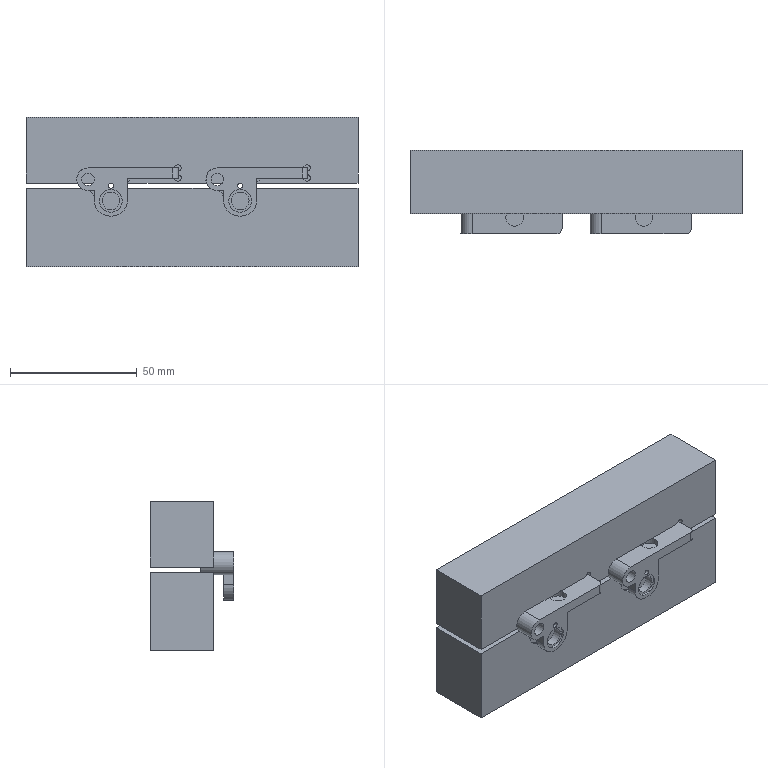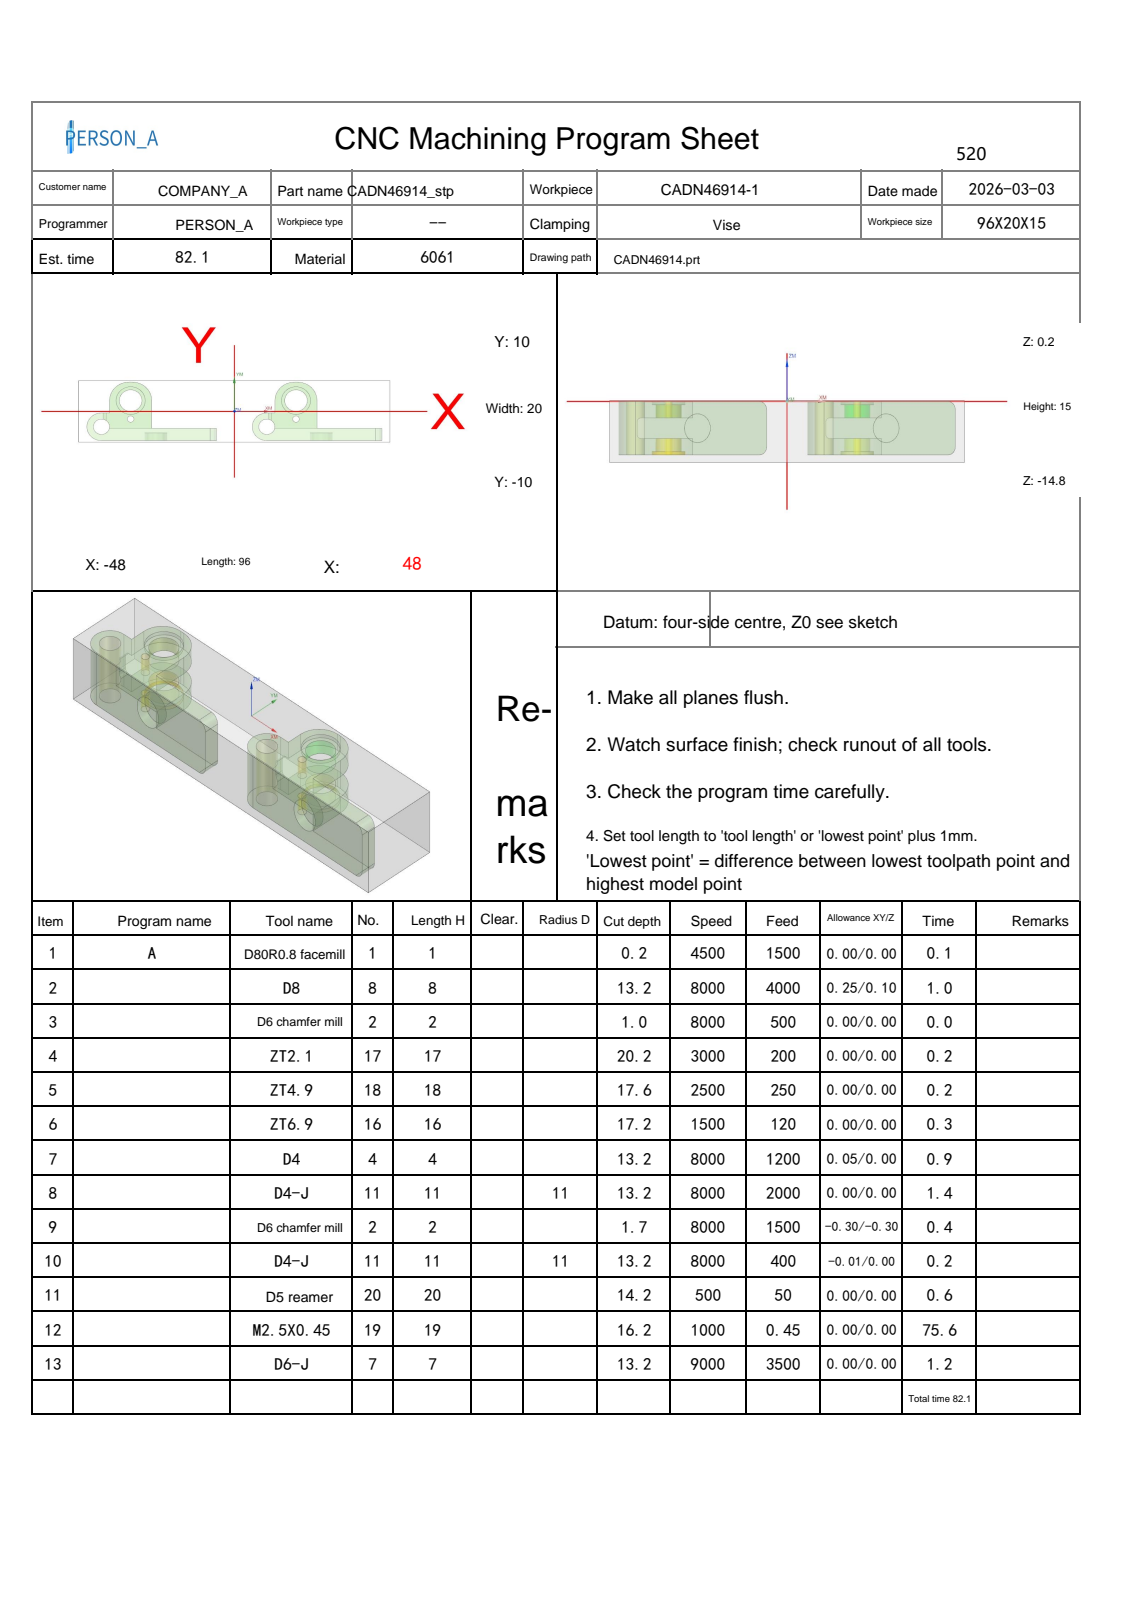NC program | NX | posted by the shop | part box 131 x 33 x 59 mm
Lines 9140 to 10309 of 12027:
N13 T07 M06
(D6-J  D=6. R=0. H=07 ce=0.01 di=0.00)
G00 G90 G54 X46.649 Y.748 M03 S7000
G43 H07 Z10.2
M08
Z.492
G01 Z-.008 F3500.
X46.545 Y-4.398
G02 X46.689 Y-5.5 I-16.56 J-2.717
G01 Y-9.5
G02 X46.536 Y-10.609 I-18.771 J2.023
G01 X46.578 Y-10.607 Z-.012
X46.729 Y-9.5
Y-5.5
G03 X46.592 Y-4.399 I-822.675 J-101.969
G01 X46.63 Y-4.4 Z-.016
G03 X46.738 Y-5.181 I4.184 J.179
G01 X46.707 Y-5.189
X46.762 Y-5.5
Y-9.5
X46.619 Y-10.601
X46.64 Y-10.6 Z-.02
X46.695 Y-10.135
X46.72 Y-10.074
X46.792 Y-9.5
Y-5.5
X46.735 Y-5.189
X46.752 Y-5.201
X46.77 Y-5.19
X46.767 Y-5.17
X46.758 Y-5.109
G02 X46.653 Y-4.4 I3.354 J.858
G01 X46.675 Z-.024
X46.674 Y-4.451
G03 X46.729 Y-4.821 I1.275 J0.0
G01 X46.715 Y-4.848
X46.75 Y-4.874
X46.802 Y-5.178
X46.764 Y-5.189
X46.819 Y-5.5
Y-9.5
G02 X46.736 Y-10.108 I-2.526 J.034
G01 X46.722 Y-10.122
X46.658 Y-10.601
X46.675 Z-.028
X46.751 Y-10.206
X46.742 Y-10.141
X46.781 Y-10.086
X46.802 Y-10.022
X46.803 Y-9.954
X46.843 Y-9.5
Y-5.5
X46.792 Y-5.189
X46.826 Y-5.177
X46.819 Y-5.167
X46.775 Y-4.873
X46.742
X46.73 Y-4.837
X46.757 Y-4.818
G02 X46.697 Y-4.449 I1.094 J.369
G01 X46.698 Y-4.4
X46.721 Z-.032
X46.719 Y-4.447
G03 X46.785 Y-4.815 I1.055 J0.0
G01 X46.754 Y-4.83
X46.761 Y-4.868
X46.795 Y-4.872
X46.839 Y-5.166
X46.849 Y-5.176
X46.82 Y-5.189
X46.866 Y-5.5
Y-9.5
G02 X46.809 Y-10.084 I-5.205 J.215
G01 X46.766 Y-10.143
X46.778 Y-10.209
X46.693 Y-10.601
X46.71 Y-10.602 Z-.036
X46.801 Y-10.211
X46.78 Y-10.188
X46.777 Y-10.157
X46.794 Y-10.13
X46.818 Y-10.117
G03 X46.888 Y-9.5 I-2.923 J.644
G01 Y-5.5
X46.849 Y-5.189
X46.858 Y-5.193
X46.865 Y-5.185
X46.861 Y-5.176
X46.815 Y-4.871
X46.783 Y-4.864
X46.777 Y-4.829
X46.805 Y-4.812
G02 X46.743 Y-4.416 I1.229 J.396
G01 Y-4.399
X46.765 Z-.038
X46.766 Z-.04
G03 X46.822 Y-4.81 I1.682 J.022
G01 X46.799 Y-4.83
X46.805 Y-4.862
X46.835 Y-4.87
G02 X46.908 Y-5.5 I-4.491 J-.843
G01 Y-9.5
G02 X46.843 Y-10.12 I-3.998 J.106
G01 X46.824 Y-10.115
X46.809 Y-10.129
X46.813 Y-10.148
X46.817 Y-10.213
X46.728 Y-10.602
X46.744 Z-.044
G03 X46.913 Y-9.785 I-8.742 J2.237
G01 X46.927 Y-9.5
Y-5.5
G03 X46.862 Y-4.936 I-2.943 J-.055
G02 X46.788 Y-4.399 I2.404 J.604
G01 X46.802 Z-.046
X46.805 Z-.048
Y-4.404
G03 X46.855 Y-4.803 I1.626 J0.0
G02 X46.946 Y-5.5 I-2.862 J-.726
G01 Y-9.5
G02 X46.761 Y-10.602 I-4.616 J.208
G01 X46.777 Z-.052
X46.895 Y-10.099
G03 X46.963 Y-9.514 I-2.488 J.584
G01 Y-5.5
G03 X46.873 Y-4.805 I-2.886 J-.021
G02 X46.82 Y-4.434 I1.262 J.371
G01 Y-4.399
X46.835 Z-.056
X46.834 Y-4.435
G03 X46.89 Y-4.803 I1.252 J0.0
G02 X46.98 Y-5.496 I-2.615 J-.693
G01 Y-5.5
Y-9.5
G02 X46.907 Y-10.159 I-3.404 J.044
G01 X46.884 Y-10.22
X46.865 Y-10.298
X46.794 Y-10.602
X46.81 Z-.06
X46.9 Y-10.222
X46.925 Y-10.145
G03 X46.996 Y-9.5 I-3.369 J.697
G01 Y-5.5
Y-5.499
G03 X46.872 Y-4.673 I-2.806 J0.0
G01 X46.85 Y-4.4
X46.865 Z-.064
X46.864 Y-4.439
G03 X46.923 Y-4.799 I1.119 J0.0
G01 X46.94 Y-4.848
G02 X47.012 Y-5.5 I-3.583 J-.726
G01 Y-9.5
G02 X46.941 Y-10.146 I-3.831 J.095
G01 X46.917 Y-10.224
X46.827 Y-10.602
X46.843 Z-.068
G03 X47.027 Y-9.5 I-4.589 J1.332
G01 Y-5.477
G03 X46.919 Y-4.724 I-2.67 J0.0
G02 X46.879 Y-4.443 I.959 J.281
G01 Y-4.4
X46.894 Z-.072
Y-4.432
G03 X46.929 Y-4.688 I.946 J0.0
G02 X47.042 Y-5.5 I-3.368 J-.881
G01 Y-9.5
G02 X46.86 Y-10.602 I-4.792 J.225
G01 X46.876 Z-.076
G03 X47.056 Y-9.5 I-4.798 J1.348
G01 Y-5.5
G03 X46.965 Y-4.765 I-4.457 J-.18
G01 X46.958 Y-4.744
G02 X46.908 Y-4.441 I.887 J.303
G01 X46.909 Y-4.4
X46.924 Z-.08
Y-4.423
G03 X46.951 Y-4.655 I.983 J0.0
G02 X47.07 Y-5.5 I-4.213 J-1.022
G01 Y-9.5
G02 X46.893 Y-10.602 I-5.338 J.293
G01 X46.909 Z-.084
G03 X47.084 Y-9.5 I-5.534 J1.439
G01 Y-5.5
G03 X46.974 Y-4.706 I-4.032 J-.151
G02 X46.939 Y-4.418 I1.159 J.289
G01 Y-4.4
X46.953 Z-.086
X46.954 Z-.088
G03 X47.006 Y-4.786 I1.493 J.003
G02 X47.097 Y-5.5 I-3.649 J-.829
G01 Y-9.5
X47.055 Y-9.957
X46.926 Y-10.602
X46.942 Y-10.601 Z-.092
X47.063 Y-9.983
G03 X47.11 Y-9.507 I-2.419 J.476
G01 Y-5.5
G03 X47.005 Y-4.745 I-3.431 J-.089
G02 X46.967 Y-4.442 I1.193 J.303
G01 X46.968 Y-4.4
X46.977 Z-.094
X46.979 Z-.096
X46.978 Y-4.444
G03 X47.017 Y-4.749 I1.188 J0.0
G02 X47.122 Y-5.5 I-3.055 J-.809
G01 Y-9.501
G02 X47.073 Y-9.999 I-2.565 J0.0
G01 X46.965 Y-10.547
X46.957 Y-10.601
X46.973 Z-.1
G02 X47.076 Y-10.038 I6.185 J-.841
G03 X47.135 Y-9.522 I-2.236 J.516
G01 Y-5.5
G03 X47.03 Y-4.753 I-2.912 J-.027
G02 X46.989 Y-4.449 I1.102 J.304
G01 X46.99 Y-4.4
X47.001 Z-.104
X46.999 Y-4.455
G03 X47.041 Y-4.754 I1.082 J0.0
G02 X47.147 Y-5.5 I-2.611 J-.749
G01 Y-9.552
G02 X47.09 Y-10.032 I-2.062 J0.0
G03 X46.985 Y-10.601 I5.359 J-1.284
G01 X46.987 Z-.106
X46.997 Z-.108
G02 X47.097 Y-10.053 I4.944 J-.626
G03 X47.158 Y-9.542 I-2.112 J.512
G01 Y-5.5
Y-5.498
G03 X47.053 Y-4.756 I-2.658 J0.0
G02 X47.01 Y-4.457 I1.027 J.299
G01 X47.012 Y-4.4
X47.023 Z-.112
X47.02 Y-4.468
G03 X47.062 Y-4.75 I.964 J0.0
G02 X47.17 Y-5.474 I-2.372 J-.724
G01 Y-5.5
Y-9.5
G02 X47.135 Y-9.957 I-4.923 J.146
G03 X47.009 Y-10.601 I4.41 J-1.201
G01 X47.021 Z-.116
G02 X47.146 Y-9.957 I4.894 J-.613
G03 X47.182 Y-9.5 I-5.306 J.652
G01 Y-5.5
G03 X47.099 Y-4.848 I-2.646 J-.007
G01 X47.097 Y-4.768
X47.057 Y-4.697
G02 X47.034 Y-4.404 I1.898 J.293
G01 Y-4.4
X47.046 Z-.121
X47.068 Y-4.696
X47.102 Y-4.776
X47.111 Y-4.848
X47.164 Y-5.135
G02 X47.194 Y-5.469 I-1.826 J-.333
G01 Y-9.51
G02 X47.13 Y-10.064 I-2.444 J0.0
G03 X47.034 Y-10.601 I5.243 J-1.219
G01 X47.047 Z-.125
G02 X47.144 Y-10.056 I5.891 J-.768
G03 X47.206 Y-9.503 I-2.442 J.553
G01 Y-5.5
Y-5.476
G03 X47.185 Y-5.189 I-1.947 J0.0
G01 X47.124 Y-4.848
X47.114 Y-4.774
X47.079 Y-4.695
X47.058 Y-4.4
X47.07 Z-.129
X47.09 Y-4.694
X47.127 Y-4.773
X47.137 Y-4.848
X47.196 Y-5.189
G02 X47.218 Y-5.475 I-1.87 J-.286
G01 Y-5.5
Y-9.505
G02 X47.158 Y-10.043 I-2.469 J0.0
G03 X47.06 Y-10.601 I6.131 J-1.369
G01 X47.071 Z-.132
X47.073 Z-.134
G02 X47.173 Y-10.029 I7.441 J-1.009
G03 X47.229 Y-9.504 I-2.438 J.525
G01 Y-5.5
Y-5.479
G03 X47.207 Y-5.189 I-1.927 J0.0
G01 X47.15 Y-4.848
X47.139 Y-4.772
X47.102 Y-4.692
X47.082 Y-4.4
X47.095 Z-.138
X47.113 Y-4.691
X47.143 Y-4.732
X47.148 Y-4.783
G02 X47.241 Y-5.5 I-3.31 J-.792
G01 Y-9.505
G02 X47.188 Y-10.015 I-2.493 J0.0
G03 X47.086 Y-10.601 I8.476 J-1.771
G01 X47.099 Z-.143
X47.143 Y-10.298
X47.171 Y-10.173
G03 X47.252 Y-9.5 I-3.724 J.788
G01 Y-5.5
G03 X47.163 Y-4.79 I-3.575 J-.086
G01 X47.157 Y-4.735
X47.124 Y-4.69
X47.107 Y-4.4
X47.119 Z-.147
X47.136 Y-4.689
X47.178 Y-4.763
X47.189 Y-4.848
G02 X47.263 Y-5.5 I-3.658 J-.745
G01 Y-9.503
G02 X47.165 Y-10.254 I-2.937 J0.0
G01 X47.154 Y-10.298
X47.112 Y-10.601
X47.126 Z-.152
X47.165 Y-10.298
X47.183 Y-10.237
G03 X47.275 Y-9.5 I-3.818 J.848
G01 Y-5.5
G03 X47.203 Y-4.848 I-3.879 J-.096
G01 X47.18 Y-4.767
X47.148 Y-4.687
G02 X47.132 Y-4.4 I3.666 J.345
G01 X47.146 Z-.157
X47.154 Y-4.638
X47.175 Y-4.712
G02 X47.287 Y-5.496 I-2.696 J-.785
G01 Y-9.5
G02 X47.195 Y-10.238 I-3.778 J.094
G01 X47.176 Y-10.298
X47.141 Y-10.6
X47.156 Z-.162
X47.188 Y-10.298
X47.208 Y-10.239
G03 X47.299 Y-9.5 I-3.54 J.813
G01 Y-5.451
G03 X47.202 Y-4.765 I-2.483 J0.0
G02 X47.158 Y-4.476 I.907 J.289
G01 X47.161 Y-4.4
X47.175 Z-.168
X47.188 Y-4.683
G02 X47.312 Y-5.475 I-2.476 J-.792
G01 X47.311 Y-5.5
Y-9.5
G02 X47.221 Y-10.24 I-3.466 J.05
G01 X47.2 Y-10.298
X47.172 Y-10.6
X47.188 Z-.173
X47.213 Y-10.298
G03 X47.324 Y-9.5 I-2.862 J.804
G01 Y-5.5
Y-5.477
G03 X47.202 Y-4.681 I-2.654 J0.0
G01 X47.19 Y-4.4
X47.205 Z-.179
X47.216 Y-4.68
G02 X47.336 Y-5.496 I-2.713 J-.816
G01 Y-5.5
Y-9.5
Y-9.508
G02 X47.226 Y-10.298 I-2.876 J0.0
G01 X47.204 Y-10.6
X47.22 Z-.184
X47.239 Y-10.298
G03 X47.349 Y-9.5 I-2.994 J.819
G01 Y-5.5
G03 X47.25 Y-4.739 I-3.274 J-.037
G02 X47.218 Y-4.479 I1.037 J.26
G01 X47.221 Y-4.4
X47.237 Z-.19
X47.235 Y-4.472
G03 X47.275 Y-4.802 I1.366 J0.0
G02 X47.361 Y-5.5 I-2.812 J-.7
G01 Y-9.5
G02 X47.269 Y-10.234 I-3.542 J.069
G03 X47.235 Y-10.533 I1.284 J-.299
G01 X47.237 Y-10.6
X47.254 Z-.196
X47.25 Y-10.511
G02 X47.28 Y-10.247 I1.194 J0.0
G03 X47.373 Y-9.5 I-3.736 J.846
G01 Y-5.5
G03 X47.284 Y-4.773 I-3.481 J-.058
G02 X47.25 Y-4.478 I1.279 J.296
G01 X47.253 Y-4.4
X47.269 Z-.202
X47.267 Y-4.478
G03 X47.302 Y-4.81 I1.582 J0.0
G02 X47.385 Y-5.5 I-3.736 J-.801
G01 Y-9.5
G02 X47.287 Y-10.276 I-4.279 J.147
G03 X47.264 Y-10.487 I.961 J-.212
G01 X47.271 Y-10.6
X47.288 Z-.208
X47.292 Y-10.298
G03 X47.398 Y-9.5 I-3.987 J.932
G01 Y-5.5
G03 X47.316 Y-4.813 I-4.303 J-.165
G02 X47.283 Y-4.487 I1.612 J.326
G01 X47.285 Y-4.4
X47.301 Z-.211
X47.306 Z-.214
X47.305 Y-4.464
G03 X47.354 Y-4.943 I2.393 J0.0
G01 X47.41 Y-5.5
Y-9.5
G02 X47.325 Y-10.2 I-4.378 J.175
G03 X47.295 Y-10.449 I1.025 J-.249
G01 X47.306 Y-10.6
X47.318 Z-.22
X47.307 Y-10.45
G02 X47.336 Y-10.201 I1.076 J0.0
G03 X47.422 Y-9.5 I-4.237 J.876
G01 Y-5.5
X47.375 Y-5.027
X47.365 Y-4.942
G02 X47.315 Y-4.421 I2.673 J.521
G01 Y-4.4
X47.324 Z-.223
X47.327 Z-.227
Y-4.428
G03 X47.377 Y-4.941 I2.639 J0.0
G01 X47.386 Y-5.026
X47.435 Y-5.5
Y-9.5
G02 X47.348 Y-10.202 I-4.222 J.167
G03 X47.319 Y-10.45 I1.07 J-.247
G01 X47.33 Y-10.6
X47.342 Z-.233
X47.332 Y-10.45
G02 X47.359 Y-10.203 I1.123 J0.0
G03 X47.447 Y-9.5 I-4.003 J.857
G01 Y-5.5
X47.397 Y-5.025
X47.389 Y-4.941
G02 X47.339 Y-4.435 I2.507 J.506
G01 Y-4.4
X47.348 Z-.236
X47.351 Z-.24
G03 X47.43 Y-5.189 I7.637 J.36
G01 X47.459 Y-5.5
Y-9.5
G02 X47.371 Y-10.204 I-3.936 J.137
G03 X47.344 Y-10.45 I1.123 J-.246
G01 X47.354 Y-10.6
X47.366 Z-.246
X47.357 Y-10.45
G02 X47.383 Y-10.205 I1.179 J0.0
G03 X47.471 Y-9.5 I-3.696 J.824
G01 Y-5.5
X47.442 Y-5.189
G02 X47.364 Y-4.4 I7.656 J1.157
G01 X47.373 Z-.25
X47.376 Z-.253
G03 X47.454 Y-5.189 I7.872 J.379
G01 X47.483 Y-5.5
Y-9.5
G02 X47.394 Y-10.206 I-3.788 J.119
G03 X47.37 Y-10.45 I1.186 J-.244
G01 X47.379 Y-10.6
X47.392 Z-.26
X47.382 Y-10.449
G02 X47.428 Y-10.118 I1.212 J0.0
X47.482 Y-9.778 I2.42 J-.208
G01 X47.496 Y-9.5
Y-5.5
X47.467 Y-5.189
G02 X47.389 Y-4.4 I7.949 J1.181
G01 X47.398 Z-.263
X47.402 Z-.267
G03 X47.508 Y-5.5 I22.285 J1.585
G01 Y-9.5
G02 X47.419 Y-10.208 I-3.811 J.119
G03 X47.396 Y-10.45 I1.263 J-.242
G01 X47.405 Y-10.6
X47.418 Z-.274
X47.409 Y-10.45
G02 X47.431 Y-10.209 I1.33 J0.0
G03 X47.52 Y-9.5 I-3.868 J.843
G01 Y-5.5
X47.493 Y-5.189
G02 X47.415 Y-4.4 I8.233 J1.205
G01 X47.425 Z-.277
X47.428 Z-.281
G03 X47.506 Y-5.189 I8.509 J.433
G01 X47.532 Y-5.5
Y-9.5
G02 X47.444 Y-10.21 I-4.097 J.147
G03 X47.423 Y-10.45 I1.358 J-.24
G01 X47.431 Y-10.6
X47.444 Z-.288
X47.437 Y-10.45
G02 X47.457 Y-10.211 I1.434 J0.0
G03 X47.544 Y-9.5 I-4.186 J.874
G01 Y-5.5
G03 X47.508 Y-5.118 I-3.844 J-.162
G02 X47.442 Y-4.4 I7.221 J1.032
G01 X47.451 Z-.291
X47.455 Z-.295
X47.483 Y-4.848
G02 X47.555 Y-5.5 I-5.164 J-.9
G01 Y-9.5
G02 X47.475 Y-10.182 I-4.26 J.155
G03 X47.449 Y-10.447 I1.327 J-.266
G01 X47.458 Y-10.6
X47.471 Z-.302
X47.464 Y-10.45
G02 X47.498 Y-10.124 I1.549 J0.0
G03 X47.567 Y-9.5 I-4.31 J.788
G01 Y-5.5
G03 X47.494 Y-4.848 I-4.534 J-.176
G01 X47.468 Y-4.4
X47.478 Z-.306
X47.481 Z-.309
X47.505 Y-4.848
G02 X47.578 Y-5.5 I-3.894 J-.768
G01 Y-9.5
G02 X47.509 Y-10.124 I-4.041 J.132
G03 X47.477 Y-10.452 I1.645 J-.328
G01 X47.483 Y-10.6
X47.491 Z-.313
X47.495 Z-.316
X47.489 Y-10.459
G02 X47.519 Y-10.141 I1.707 J0.0
G03 X47.589 Y-9.5 I-4.09 J.774
G01 Y-5.5
G03 X47.516 Y-4.848 I-3.503 J-.067
G01 X47.493 Y-4.4
X47.504 Z-.32
X47.505 Z-.323
X47.526 Y-4.848
G02 X47.6 Y-5.5 I-3.043 J-.676
G01 Y-9.5
G02 X47.529 Y-10.16 I-4.302 J.133
G03 X47.501 Y-10.462 I1.611 J-.302
G01 X47.506 Y-10.6
X47.518 Z-.327
Z-.331
X47.514 Y-10.465
G02 X47.541 Y-10.127 I2.111 J0.0
G01 X47.562 Y-10.042
X47.576 Y-9.957
X47.612 Y-9.5
Y-5.5
G03 X47.537 Y-4.848 I-2.966 J-.008
G01 X47.518 Y-4.4
X47.532 Z-.335
X47.531 Z-.339
X47.549 Y-4.848
G02 X47.623 Y-5.5 I-2.832 J-.652
G01 Y-9.5
X47.588 Y-9.957
X47.574 Y-10.043
X47.553 Y-10.128
G03 X47.529 Y-10.495 I2.818 J-.367
G01 X47.531 Y-10.6
X47.547 Z-.343
X47.544 Z-.347
X47.541 Y-10.488
G02 X47.585 Y-10.044 I2.294 J0.0
G03 X47.635 Y-9.5 I-3.445 J.594
G01 Y-5.5
Y-5.498
G03 X47.561 Y-4.848 I-2.89 J0.0
G01 X47.545 Y-4.4
X47.562 Z-.351
X47.558 Z-.355
X47.574 Y-4.848
G02 X47.647 Y-5.492 I-2.784 J-.644
G01 Y-5.5
Y-9.5
G02 X47.596 Y-10.045 I-3.149 J.019
G03 X47.554 Y-10.481 I2.235 J-.436
G01 X47.557 Y-10.6
X47.577 Z-.359
X47.57 Z-.363
X47.566 Y-10.462
G02 X47.608 Y-10.046 I2.093 J0.0
G03 X47.659 Y-9.5 I-2.945 J.551
G01 Y-5.5
Y-5.49
G03 X47.586 Y-4.848 I-2.859 J0.0
G01 X47.571 Y-4.4
X47.593 Z-.367
X47.584 Z-.371
X47.598 Y-4.848
G02 X47.671 Y-5.498 I-2.891 J-.65
G01 Y-5.5
Y-9.5
G02 X47.619 Y-10.047 I-3.063 J.011
G03 X47.579 Y-10.456 I2.04 J-.409
G01 X47.584 Y-10.6
X47.601 Z-.375
X47.597 Z-.38
X47.592 Y-10.451
G02 X47.63 Y-10.056 I2.112 J0.0
G03 X47.682 Y-9.5 I-2.931 J.558
G01 Y-5.5
G03 X47.611 Y-4.848 I-3.037 J-.002
G01 X47.597 Y-4.4
X47.612 Z-.384
X47.61 Z-.388
X47.624 Y-4.848
G02 X47.694 Y-5.5 I-3.126 J-.666
G01 Y-9.5
G02 X47.627 Y-10.133 I-3.125 J.012
G01 X47.618 Y-10.223
X47.611 Y-10.6
X47.624 Z-.392
X47.625 Z-.397
X47.63 Y-10.224
X47.639 Y-10.134
X47.648 Y-10.089
G03 X47.706 Y-9.5 I-3.167 J.608
G01 Y-5.5
G03 X47.648 Y-4.909 I-3.186 J-.014
G01 X47.637 Y-4.848
X47.623 Y-4.4
X47.636 Z-.401
X47.637 Z-.405
X47.65 Y-4.848
G02 X47.717 Y-5.5 I-3.677 J-.711
G01 Y-9.5
G02 X47.667 Y-10.05 I-3.216 J.018
G03 X47.633 Y-10.431 I2.127 J-.381
G01 X47.639 Y-10.6
X47.652 Z-.414
X47.647 Y-10.436
G02 X47.686 Y-9.998 I2.44 J0.0
G01 X47.694 Y-9.957
G03 X47.729 Y-9.5 I-3.387 J.489
G01 Y-5.5
G03 X47.66 Y-4.848 I-3.759 J-.065
G01 X47.65 Y-4.4
X47.66 Z-.423
X47.671 Y-4.848
G02 X47.74 Y-5.5 I-3.713 J-.723
G01 Y-9.5
G02 X47.705 Y-9.957 I-3.3 J.025
G01 X47.697 Y-9.998
G03 X47.657 Y-10.436 I2.384 J-.438
G01 X47.663 Y-10.6
X47.674 Z-.432
X47.667 Y-10.426
G02 X47.704 Y-10.021 I2.234 J0.0
G03 X47.751 Y-9.504 I-2.8 J.517
G01 Y-5.5
G03 X47.682 Y-4.848 I-3.784 J-.074
G01 X47.671 Y-4.4
X47.68 Z-.436
X47.682 Z-.441
X47.693 Y-4.848
G02 X47.763 Y-5.5 I-3.696 J-.726
G01 Y-9.508
G02 X47.716 Y-10.018 I-2.794 J0.0
G03 X47.678 Y-10.427 I2.205 J-.409
G01 X47.685 Y-10.6
X47.696 Z-.45
X47.689 Y-10.426
G02 X47.727 Y-10.02 I2.212 J0.0
G03 X47.774 Y-9.508 I-2.741 J.512
G01 Y-5.5
G03 X47.704 Y-4.848 I-3.763 J-.075
G01 X47.693 Y-4.4
X47.702 Z-.455
X47.705 Z-.459
X47.715 Y-4.848
G02 X47.785 Y-5.5 I-3.694 J-.726
G01 Y-9.5
G02 X47.75 Y-9.957 I-3.35 J.029
G01 X47.742 Y-9.999
G03 X47.701 Y-10.435 I2.321 J-.436
G01 X47.707 Y-10.6
X47.719 Z-.469
X47.713 Y-10.435
G02 X47.754 Y-10. I2.348 J0.0
G01 X47.762 Y-9.957
G03 X47.796 Y-9.5 I-3.522 J.499
G01 Y-5.5
G03 X47.727 Y-4.848 I-3.745 J-.072
G01 X47.716 Y-4.4
X47.724 Z-.473
X47.727 Z-.478
X47.738 Y-4.848
G02 X47.808 Y-5.5 I-3.637 J-.717
G01 Y-9.5
G02 X47.761 Y-10.024 I-3.402 J.035
G03 X47.722 Y-10.422 I2.005 J-.398
G01 X47.73 Y-10.6
X47.742 Z-.488
X47.739 Y-10.451
G02 X47.752 Y-10.129 I3.823 J0.0
G01 X47.761 Y-10.083
G03 X47.819 Y-9.5 I-3.232 J.611
G01 Y-5.5
G03 X47.75 Y-4.848 I-3.649 J-.057
G01 X47.739 Y-4.4
X47.748 Z-.492
X47.751 Z-.497
X47.761 Y-4.848
G02 X47.83 Y-5.5 I-3.506 J-.697
G01 Y-9.5
G02 X47.795 Y-9.957 I-3.649 J.049
G01 X47.78 Y-10.048
G03 X47.748 Y-10.438 I2.364 J-.39
G01 X47.753 Y-10.6
X47.765 Z-.507
X47.761 Y-10.451
G02 X47.805 Y-9.957 I2.784 J0.0
G03 X47.84 Y-9.5 I-3.341 J.489
G01 Y-5.5
G03 X47.773 Y-4.848 I-3.619 J-.045
G01 X47.762 Y-4.4
X47.771 Z-.511
X47.774 Z-.516
X47.785 Y-4.848
G02 X47.851 Y-5.5 I-3.678 J-.704
G01 Y-9.5
G02 X47.815 Y-9.957 I-3.105 J.013
G03 X47.773 Y-10.451 I2.838 J-.494
G01 X47.777 Y-10.6
X47.789 Z-.526
X47.785 Y-10.451
G02 X47.826 Y-9.957 I2.986 J0.0
G03 X47.862 Y-9.5 I-2.991 J.465
G01 Y-5.5
G03 X47.797 Y-4.848 I-3.999 J-.071
G01 X47.786 Y-4.4
X47.795 Z-.531
X47.798 Z-.536
X47.809 Y-4.848
G02 X47.873 Y-5.5 I-4.267 J-.747
G01 Y-9.5
G02 X47.837 Y-9.957 I-2.92 J0.0
G03 X47.797 Y-10.451 I3.061 J-.494
G01 X47.801 Y-10.6
X47.813 Z-.546
X47.809 Y-10.451
G02 X47.847 Y-9.957 I3.227 J0.0
G03 X47.883 Y-9.5 I-3.007 J.466
G01 Y-5.5
G03 X47.821 Y-4.848 I-4.752 J-.127
G01 X47.81 Y-4.4
X47.819 Z-.551
X47.822 Z-.556
X47.832 Y-4.848
G02 X47.894 Y-5.5 I-5.024 J-.804
G01 Y-9.5
X47.858 Y-9.957
X47.825 Y-10.298
Y-10.6
X47.837 Z-.566
X47.834 Y-10.46
G02 X47.869 Y-9.957 I3.616 J0.0
G01 X47.875 Y-9.911
X47.905 Y-9.5
Y-5.492
G03 X47.882 Y-5.169 I-2.285 J0.0
G02 X47.833 Y-4.489 I4.758 J.68
G01 X47.834 Y-4.4
X47.844 Z-.571
X47.846 Y-4.399 Z-.577
X47.845 Y-4.472
G03 X47.875 Y-5.041 I5.494 J0.0
G01 X47.899 Y-5.189
X47.915 Y-5.5
Y-9.5
X47.849 Y-10.361
X47.845 Y-10.484
X47.849 Y-10.6
X47.857 Z-.582
X47.861 Z-.587
G02 X47.925 Y-9.5 I12.072 J-.155
G01 Y-5.5
X47.909 Y-5.189
X47.885 Y-5.04
G02 X47.858 Y-4.447 I6.408 J.593
G01 Y-4.399
X47.869 Z-.592
X47.87 Z-.597
Y-4.412
G03 X47.895 Y-5.04 I7.791 J0.0
G01 X47.919 Y-5.189
X47.936 Y-5.5
Y-9.5
G03 X47.873 Y-10.6 I11.879 J-1.227
G01 X47.882 Z-.603
X47.885 Z-.608
G02 X47.946 Y-9.5 I9.979 J-.001
G01 Y-5.5
X47.929 Y-5.189
X47.905 Y-5.039
G02 X47.882 Y-4.399 I9.882 J.681
G01 X47.894 Z-.619
G03 X47.916 Y-5.038 I11.677 J.071
G02 X47.956 Y-5.476 I-2.326 J-.438
G01 Y-5.5
Y-9.5
G03 X47.897 Y-10.5 I8.349 J-1.
G01 Y-10.6
X47.9 Z-.624
X47.908 Z-.629
X47.901 Y-10.411
G02 X47.91 Y-10.193 I2.684 J0.0
G01 X47.966 Y-9.5
Y-5.5
X47.949 Y-5.189
X47.926 Y-5.038
G02 X47.905 Y-4.444 I8.425 J.594
G01 Y-4.399
X47.914 Y-4.4 Z-.64
Y-4.489
G03 X47.936 Y-5.037 I6.699 J0.0
G01 X47.959 Y-5.189
X47.977 Y-5.5
Y-9.5
X47.918 Y-10.213
G03 X47.91 Y-10.419 I2.518 J-.205
G01 X47.917 Y-10.6
X47.926 Z-.651
X47.918 Y-10.426
X47.925 Y-10.263
X47.986 Y-9.5
Y-5.5
X47.969 Y-5.189
X47.947 Y-5.037
G02 X47.922 Y-4.507 I5.727 J.53
G01 X47.923 Y-4.4
X47.932 Z-.662
X47.939 Y-4.848
G02 X47.996 Y-5.5 I-7.149 J-.96
G01 Y-9.5
X47.931 Y-10.31
X47.926 Y-10.438
X47.935 Y-10.6
X47.944 Z-.673
X47.936 Y-10.448
X47.94 Y-10.333
X48.006 Y-9.5
Y-5.5
G03 X47.948 Y-4.848 I-5.915 J-.202
G01 X47.941 Y-4.4
X47.95 Z-.684
X47.957 Y-4.848
X47.965 Y-4.937
X47.979 Y-5.035
G02 X48.016 Y-5.5 I-3.182 J-.489
G01 Y-9.5
X47.989 Y-9.871
X47.964 Y-10.119
G03 X47.948 Y-10.431 I3.065 J-.312
G01 X47.953 Y-10.6
X47.962 Z-.695
X47.956 Y-10.459
X47.961 Y-10.328
X48.026 Y-9.5
Y-5.5
G03 X47.966 Y-4.848 I-6.113 J-.231
G01 X47.96 Y-4.4
X47.969 Z-.706
X47.975 Y-4.848
G02 X48.035 Y-5.5 I-6.644 J-.94
G01 Y-9.5
X47.97 Y-10.331
X47.965 Y-10.456
X47.971 Y-10.6
X47.981 Z-.718
X47.978 Y-10.441
G02 X47.997 Y-10.026 I4.576 J0.0
G01 X48.045 Y-9.5
Y-5.5
G03 X47.985 Y-4.848 I-6.606 J-.282
G01 X47.978 Y-4.4
X47.986 Z-.723
X47.989 Z-.729
X47.994 Y-4.848
G02 X48.054 Y-5.5 I-6.651 J-.947
G01 Y-9.5
G03 X47.99 Y-10.6 I9.641 J-1.114
G01 X47.999 Z-.74
Y-10.593
G02 X48.064 Y-9.5 I9.33 J0.0
G01 Y-5.5
G03 X48.002 Y-4.848 I-6.938 J-.323
G01 X47.996 Y-4.4
X48.005 Z-.752
X48.011 Y-4.848
G02 X48.073 Y-5.5 I-7.049 J-.995
G01 Y-9.5
G03 X48.009 Y-10.573 I8.942 J-1.073
G01 Y-10.6
X48.018 Z-.764
Y-10.554
G02 X48.082 Y-9.5 I8.726 J0.0
G01 Y-5.5
G03 X48.02 Y-4.848 I-7.221 J-.357
G01 X48.015 Y-4.4
X48.024 Z-.775
X48.029 Y-4.848
G02 X48.091 Y-5.5 I-7.2 J-1.014
G01 Y-9.5
G03 X48.028 Y-10.537 I8.42 J-1.037
G01 Y-10.6
X48.037 Z-.787
Y-10.521
G02 X48.1 Y-9.5 I8.275 J0.0
G01 Y-5.5
G03 X48.038 Y-4.848 I-7.233 J-.36
G01 X48.033 Y-4.4
X48.039 Z-.799
X48.044 Y-4.848
G02 X48.106 Y-5.5 I-7.112 J-1.005
G01 Y-9.5
X48.049 Y-10.168
G03 X48.038 Y-10.421 I2.964 J-.253
G01 X48.044 Y-10.6
X48.052 Z-.805
X48.057 Z-.811
X48.051 Y-10.416
G02 X48.061 Y-10.176 I2.845 J0.0
G01 X48.118 Y-9.5
Y-5.5
G03 X48.056 Y-4.848 I-6.971 J-.331
G01 X48.052 Y-4.4
X48.061 Z-.823
X48.066 Y-4.848
G02 X48.127 Y-5.5 I-6.692 J-.958
G01 Y-9.5
X48.07 Y-10.176
G03 X48.06 Y-10.413 I2.84 J-.238
G01 X48.066 Y-10.6
X48.076 Z-.835
X48.07 Y-10.41
G02 X48.079 Y-10.189 I2.693 J0.0
G01 X48.135 Y-9.5
Y-5.5
G03 X48.075 Y-4.848 I-6.49 J-.276
G01 X48.071 Y-4.4
X48.08 Z-.847
X48.084 Y-4.848
G02 X48.144 Y-5.5 I-6.134 J-.893
G01 Y-9.5
X48.087 Y-10.205
G03 X48.079 Y-10.408 I2.499 J-.202
G01 X48.086 Y-10.6
X48.096 Z-.859
X48.088 Y-10.407
X48.096 Y-10.219
X48.153 Y-9.5
Y-5.5
G03 X48.093 Y-4.848 I-5.876 J-.205
G01 X48.09 Y-4.4
X48.099 Z-.871
X48.103 Y-4.848
G02 X48.161 Y-5.5 I-5.489 J-.819
G01 Y-9.5
X48.103 Y-10.251
X48.097 Y-10.408
X48.106 Y-10.599
X48.116 Z-.884
X48.105 Y-10.417
X48.109 Y-10.304
X48.169 Y-9.5
Y-5.5
G03 X48.112 Y-4.848 I-5.215 J-.129
G01 X48.109 Y-4.4
X48.119 Z-.896
X48.122 Y-4.848
G02 X48.178 Y-5.5 I-5.036 J-.76
G01 Y-9.5
X48.118 Y-10.322
X48.115 Y-10.429
X48.124 Y-10.599
X48.133 Y-10.6 Z-.908
X48.124 Y-10.443
X48.128 Y-10.343
X48.186 Y-9.5
Y-5.5
G03 X48.131 Y-4.848 I-5.802 J-.157
G01 X48.128 Y-4.4
X48.137 Z-.921
X48.141 Y-4.848
G02 X48.194 Y-5.5 I-6.639 J-.868
G01 Y-9.5
X48.138 Y-10.324
X48.134 Y-10.441
X48.141 Y-10.6
X48.149 Z-.933
X48.146 Y-10.43
G02 X48.155 Y-10.153 I3.899 J0.0
G01 X48.202 Y-9.5
Y-5.5
G03 X48.151 Y-4.848 I-7.833 J-.289
G01 X48.146 Y-4.399
X48.155 Z-.946
X48.16 Y-4.848
G02 X48.21 Y-5.5 I-9.195 J-1.028
G01 Y-9.5
G03 X48.158 Y-10.6 I11.718 J-1.105
G01 X48.165 Z-.959
G02 X48.218 Y-9.5 I12.247 J-.035
G01 Y-5.5
G03 X48.167 Y-4.848 I-8.543 J-.339
G01 X48.162 Y-4.399
X48.169 Z-.972
X48.173 Y-4.848
G02 X48.225 Y-5.5 I-7.807 J-.951
G01 Y-9.5
X48.19 Y-9.957
G03 X48.17 Y-10.446 I5.968 J-.489
G01 X48.172 Y-10.6
X48.179 Z-.984
X48.176 Y-10.442
G02 X48.197 Y-9.957 I5.842 J0.0
G01 X48.233 Y-9.5
Y-5.5
G03 X48.18 Y-4.848 I-7.208 J-.258
G01 X48.175 Y-4.399
X48.182 Z-.997
X48.187 Y-4.848
G02 X48.24 Y-5.5 I-6.545 J-.869
G01 Y-9.508
G02 X48.226 Y-9.738 I-1.877 J0.0
G03 X48.183 Y-10.438 I5.658 J-.7
G01 X48.185 Y-10.6
X48.192 Z-1.01
X48.19 Y-10.435
G02 X48.233 Y-9.739 I5.567 J0.0
G03 X48.248 Y-9.509 I-1.825 J.23
G01 Y-5.5
G03 X48.193 Y-4.848 I-6.036 J-.178
G01 X48.189 Y-4.4
X48.196 Z-1.023
X48.2 Y-4.848
G02 X48.255 Y-5.5 I-5.467 J-.792
G01 Y-9.509
G02 X48.24 Y-9.743 I-1.853 J0.0
G03 X48.197 Y-10.431 I5.395 J-.688
G01 X48.199 Y-10.6
X48.206 Z-1.036
X48.203 Y-10.428
G02 X48.247 Y-9.749 I5.315 J0.0
G03 X48.262 Y-9.508 I-1.868 J.241
G01 Y-5.5
G03 X48.207 Y-4.848 I-5.165 J-.114
G01 X48.202 Y-4.4
X48.209 Z-1.049
X48.213 Y-4.848
G02 X48.27 Y-5.5 I-5.397 J-.793
G01 Y-9.507
G02 X48.253 Y-9.756 I-1.934 J0.0
G03 X48.21 Y-10.425 I5.154 J-.669
G01 X48.213 Y-10.6
X48.22 Z-1.062
X48.217 Y-10.422
G02 X48.26 Y-9.763 I5.083 J0.0
G03 X48.277 Y-9.506 I-1.968 J.257
G01 Y-5.5
G03 X48.22 Y-4.848 I-5.734 J-.168
G01 X48.216 Y-4.4
X48.223 Z-1.076
X48.227 Y-4.848
G02 X48.284 Y-5.5 I-5.947 J-.844
G01 Y-9.5
X48.245 Y-9.957
G03 X48.224 Y-10.419 I4.953 J-.462
G01 X48.227 Y-10.6
X48.234 Z-1.089
X48.231 Y-10.416
G02 X48.252 Y-9.957 I4.869 J0.0
G01 X48.29 Y-9.5
Y-5.5
G03 X48.234 Y-4.848 I-6.251 J-.214
G01 X48.23 Y-4.4
X48.237 Z-1.102
X48.241 Y-4.848
G02 X48.297 Y-5.5 I-6.414 J-.883
G01 Y-9.5
X48.26 Y-9.957
G03 X48.238 Y-10.414 I4.746 J-.457
G01 X48.241 Y-10.6
X48.248 Z-1.116
X48.245 Y-10.414
G02 X48.267 Y-9.957 I4.717 J0.0
G01 X48.304 Y-9.5
Y-5.5
G03 X48.248 Y-4.848 I-6.651 J-.244
G01 X48.244 Y-4.4
X48.251 Z-1.129
X48.255 Y-4.848
G02 X48.31 Y-5.5 I-6.731 J-.904
G01 Y-9.5
X48.274 Y-9.957
G03 X48.251 Y-10.417 I4.691 J-.46
G01 X48.255 Y-10.6
X48.262 Z-1.143
X48.258 Y-10.42
G02 X48.297 Y-9.816 I4.711 J0.0
G03 X48.317 Y-9.512 I-2.348 J.304
G01 Y-5.5
G03 X48.262 Y-4.848 I-6.871 J-.254
G01 X48.258 Y-4.4
X48.265 Z-1.156
X48.269 Y-4.848
G02 X48.323 Y-5.5 I-6.844 J-.902
G01 Y-9.501
G02 X48.302 Y-9.833 I-2.649 J0.0
G03 X48.265 Y-10.423 I4.671 J-.59
G01 X48.269 Y-10.6
X48.275 Z-1.17
X48.272 Y-10.426
G02 X48.309 Y-9.842 I4.705 J0.0
G03 X48.329 Y-9.508 I-2.667 J.334
G01 Y-5.5
G03 X48.276 Y-4.848 I-6.87 J-.24
G01 X48.272 Y-4.4
X48.279 Z-1.183
X48.283 Y-4.848
G02 X48.336 Y-5.5 I-6.014 J-.817
G01 Y-9.5
G02 X48.303 Y-9.957 I-3.845 J.046
G03 X48.279 Y-10.43 I4.679 J-.473
G01 X48.282 Y-10.6
X48.289 Z-1.197
X48.285 Y-10.438
G02 X48.293 Y-10.205 I3.39 J0.0
G01 X48.342 Y-9.5
Y-5.5
X48.325 Y-5.189
X48.29 Y-4.848
X48.286 Y-4.4
X48.293 Z-1.211
X48.297 Y-4.848
X48.331 Y-5.178
X48.348 Y-5.5
Y-9.5
X48.295 Y-10.298
X48.29 Y-10.443
X48.296 Y-10.6
X48.303 Z-1.224
X48.298 Y-10.456
X48.302 Y-10.329
X48.353 Y-9.5
Y-5.5
X48.331 Y-5.109
X48.304 Y-4.848
X48.3 Y-4.4
X48.307 Z-1.238
X48.311 Y-4.848
X48.331 Y-5.039
X48.359 Y-5.5
Y-9.5
G03 X48.31 Y-10.533 I10.712 J-1.033
G01 Y-10.6
X48.317 Z-1.252
Y-10.591
G02 X48.365 Y-9.5 I12.369 J0.0
G01 Y-5.5
X48.314 Y-4.705
X48.309 Y-4.556
X48.314 Y-4.4
X48.32 Z-1.266
G03 X48.37 Y-5.5 I13.39 J.059
G01 Y-9.5
G03 X48.323 Y-10.503 I10.64 J-1.003
G01 X48.324 Y-10.6
X48.331 Y-10.601 Z-1.28
Y-10.515
G02 X48.376 Y-9.5 I11.389 J0.0